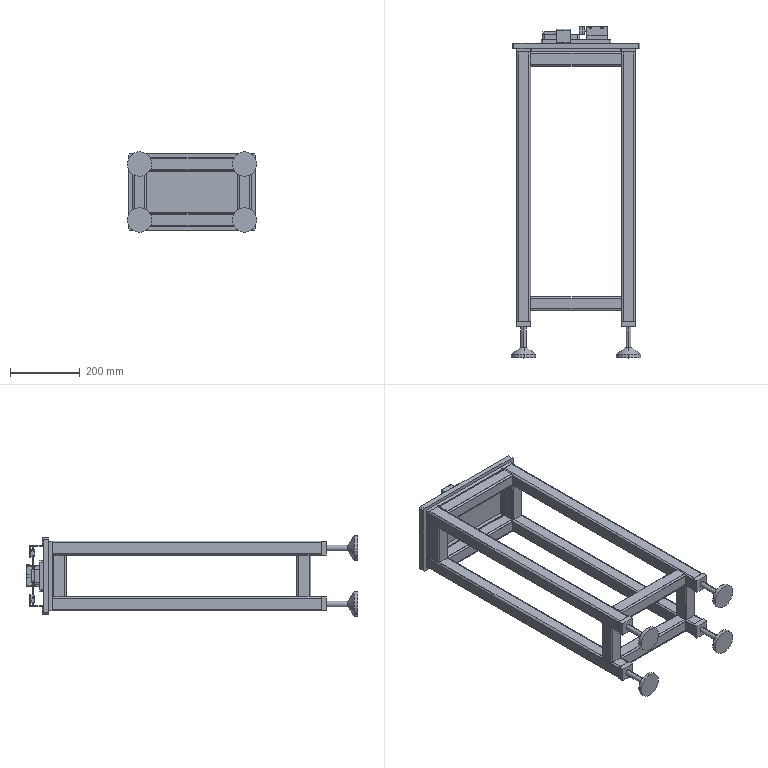Part | SolidWorks | 40 solids | 1205 faces | box 370 x 949.5 x 230 mm | volume 4110556 mm3 | plane 604 | cylinder 447 | cone 142 | spline 12 | commonest cylinder face diameters 5 x52 10 x52 0.3 x50 0.5 x44 6 x40 3 x26